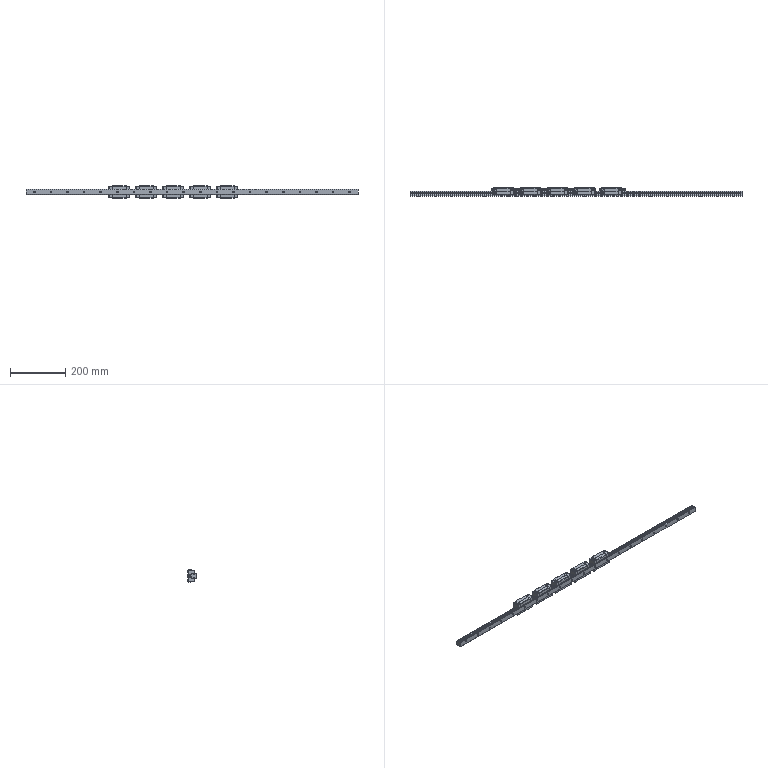Part | SolidWorks | 36 solids | 3938 faces | volume 680804 mm3 | plane 2457 | cylinder 1176 | cone 230 | spline 30 | sphere 30 | torus 15 | commonest cylinder face diameters 1 x352 0.2 x170 2 x140 4.06 x104 0.1 x90 6 x60